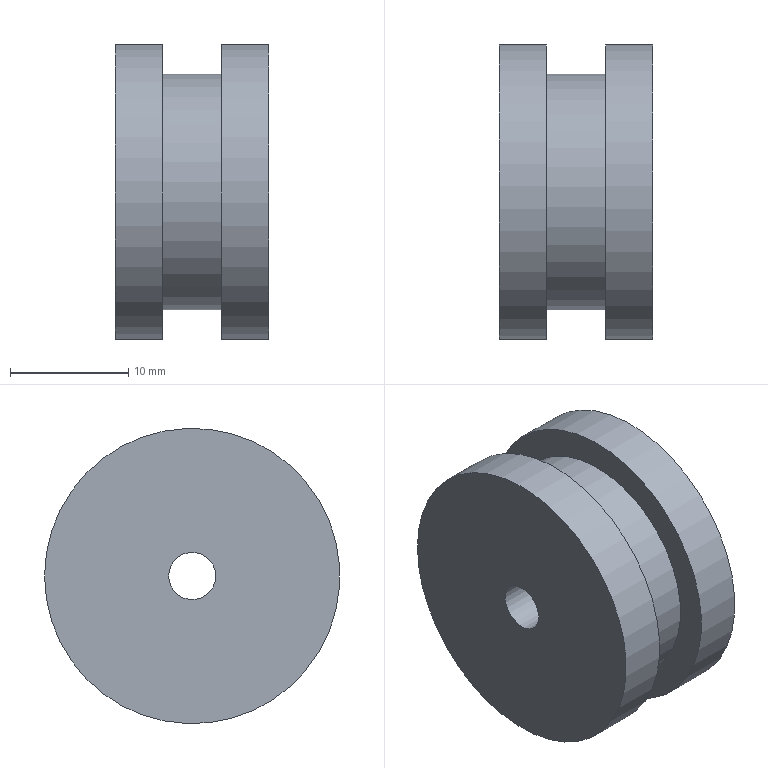Part | STEP file | 2-06.1 | 1 solid | 10 faces | box 13 x 25 x 25 mm | volume 5232 mm3 | cylinder 5 | plane 5 | commonest cylinder face diameters 25 x2 4 x1 6 x1 20 x1
STEP:
#1=CARTESIAN_POINT('',(0.,0.,0.));
#2=DIRECTION('',(0.,0.,1.));
#3=DIRECTION('',(1.,0.,0.));
#4=AXIS2_PLACEMENT_3D('',#1,#2,#3);
#5=CARTESIAN_POINT('',(2.5,10.,0.));
#6=VERTEX_POINT('',#5);
#7=CARTESIAN_POINT('',(-2.5,10.,0.));
#8=VERTEX_POINT('',#7);
#9=CARTESIAN_POINT('',(2.5,10.,0.));
#10=DIRECTION('',(-1.,0.,0.));
#11=VECTOR('',#10,1.);
#12=LINE('',#9,#11);
#13=CARTESIAN_POINT('',(2.5,0.,0.));
#14=DIRECTION('',(-1.,0.,0.));
#15=DIRECTION('',(0.,1.,0.));
#16=AXIS2_PLACEMENT_3D('',#13,#14,#15);
#17=CYLINDRICAL_SURFACE('',#16,10.);
#18=CARTESIAN_POINT('',(6.283,0.));
#19=DIRECTION('',(0.,1.));
#20=VECTOR('',#19,1.);
#21=LINE('',#18,#20);
#22=(GEOMETRIC_REPRESENTATION_CONTEXT(2)PARAMETRIC_REPRESENTATION_CONTEXT()REPRESENTATION_CONTEXT('',''));
#23=DEFINITIONAL_REPRESENTATION('',(#21),#22);
#24=PCURVE('',#17,#23);
#25=CARTESIAN_POINT('',(0.,0.));
#26=DIRECTION('',(0.,1.));
#27=VECTOR('',#26,1.);
#28=LINE('',#25,#27);
#29=(GEOMETRIC_REPRESENTATION_CONTEXT(2)PARAMETRIC_REPRESENTATION_CONTEXT()REPRESENTATION_CONTEXT('',''));
#30=DEFINITIONAL_REPRESENTATION('',(#28),#29);
#31=PCURVE('',#17,#30);
#32=SEAM_CURVE('',#12,(#24,#31),.PCURVE_S1.);
#33=EDGE_CURVE('',#6,#8,#32,.T.);
#34=ORIENTED_EDGE('',*,*,#33,.T.);
#35=CARTESIAN_POINT('',(-2.5,0.,0.));
#36=DIRECTION('',(1.,0.,0.));
#37=DIRECTION('',(0.,1.,0.));
#38=AXIS2_PLACEMENT_3D('',#35,#36,#37);
#39=CIRCLE('',#38,10.);
#40=CARTESIAN_POINT('',(6.283,5.));
#41=DIRECTION('',(-1.,0.));
#42=VECTOR('',#41,1.);
#43=LINE('',#40,#42);
#44=(GEOMETRIC_REPRESENTATION_CONTEXT(2)PARAMETRIC_REPRESENTATION_CONTEXT()REPRESENTATION_CONTEXT('',''));
#45=DEFINITIONAL_REPRESENTATION('',(#43),#44);
#46=PCURVE('',#17,#45);
#47=CARTESIAN_POINT('',(-2.5,-3.349,0.));
#48=DIRECTION('',(1.,0.,0.));
#49=DIRECTION('',(0.,0.,-1.));
#50=AXIS2_PLACEMENT_3D('',#47,#48,#49);
#51=PLANE('',#50);
#52=CARTESIAN_POINT('',(0.,3.349));
#53=DIRECTION('',(0.,1.));
#54=AXIS2_PLACEMENT_2D('',#52,#53);
#55=CIRCLE('',#54,10.);
#56=(GEOMETRIC_REPRESENTATION_CONTEXT(2)PARAMETRIC_REPRESENTATION_CONTEXT()REPRESENTATION_CONTEXT('',''));
#57=DEFINITIONAL_REPRESENTATION('',(#55),#56);
#58=PCURVE('',#51,#57);
#59=SURFACE_CURVE('',#39,(#46,#58),.PCURVE_S1.);
#60=EDGE_CURVE('',#8,#8,#59,.T.);
#61=ORIENTED_EDGE('',*,*,#60,.T.);
#62=ORIENTED_EDGE('',*,*,#33,.F.);
#63=CARTESIAN_POINT('',(2.5,0.,0.));
#64=DIRECTION('',(1.,0.,0.));
#65=DIRECTION('',(0.,1.,0.));
#66=AXIS2_PLACEMENT_3D('',#63,#64,#65);
#67=CIRCLE('',#66,10.);
#68=CARTESIAN_POINT('',(6.283,0.));
#69=DIRECTION('',(-1.,0.));
#70=VECTOR('',#69,1.);
#71=LINE('',#68,#70);
#72=(GEOMETRIC_REPRESENTATION_CONTEXT(2)PARAMETRIC_REPRESENTATION_CONTEXT()REPRESENTATION_CONTEXT('',''));
#73=DEFINITIONAL_REPRESENTATION('',(#71),#72);
#74=PCURVE('',#17,#73);
#75=CARTESIAN_POINT('',(2.5,-3.349,0.));
#76=DIRECTION('',(1.,0.,0.));
#77=DIRECTION('',(0.,0.,-1.));
#78=AXIS2_PLACEMENT_3D('',#75,#76,#77);
#79=PLANE('',#78);
#80=CARTESIAN_POINT('',(0.,3.349));
#81=DIRECTION('',(0.,1.));
#82=AXIS2_PLACEMENT_2D('',#80,#81);
#83=CIRCLE('',#82,10.);
#84=(GEOMETRIC_REPRESENTATION_CONTEXT(2)PARAMETRIC_REPRESENTATION_CONTEXT()REPRESENTATION_CONTEXT('',''));
#85=DEFINITIONAL_REPRESENTATION('',(#83),#84);
#86=PCURVE('',#79,#85);
#87=SURFACE_CURVE('',#67,(#74,#86),.PCURVE_S1.);
#88=EDGE_CURVE('',#6,#6,#87,.T.);
#89=ORIENTED_EDGE('',*,*,#88,.F.);
#90=EDGE_LOOP('',(#34,#61,#62,#89));
#91=FACE_BOUND('',#90,.T.);
#92=ADVANCED_FACE('',(#91),#17,.T.);
#93=CARTESIAN_POINT('',(-2.5,12.5,0.));
#94=VERTEX_POINT('',#93);
#95=CARTESIAN_POINT('',(-2.5,0.,0.));
#96=DIRECTION('',(1.,0.,0.));
#97=DIRECTION('',(0.,1.,0.));
#98=AXIS2_PLACEMENT_3D('',#95,#96,#97);
#99=CIRCLE('',#98,12.5);
#100=CARTESIAN_POINT('',(0.,3.349));
#101=DIRECTION('',(0.,1.));
#102=AXIS2_PLACEMENT_2D('',#100,#101);
#103=CIRCLE('',#102,12.5);
#104=(GEOMETRIC_REPRESENTATION_CONTEXT(2)PARAMETRIC_REPRESENTATION_CONTEXT()REPRESENTATION_CONTEXT('',''));
#105=DEFINITIONAL_REPRESENTATION('',(#103),#104);
#106=PCURVE('',#51,#105);
#107=CARTESIAN_POINT('',(-2.5,0.,0.));
#108=DIRECTION('',(-1.,0.,0.));
#109=DIRECTION('',(0.,1.,0.));
#110=AXIS2_PLACEMENT_3D('',#107,#108,#109);
#111=CYLINDRICAL_SURFACE('',#110,12.5);
#112=CARTESIAN_POINT('',(6.283,0.));
#113=DIRECTION('',(-1.,0.));
#114=VECTOR('',#113,1.);
#115=LINE('',#112,#114);
#116=(GEOMETRIC_REPRESENTATION_CONTEXT(2)PARAMETRIC_REPRESENTATION_CONTEXT()REPRESENTATION_CONTEXT('',''));
#117=DEFINITIONAL_REPRESENTATION('',(#115),#116);
#118=PCURVE('',#111,#117);
#119=SURFACE_CURVE('',#99,(#106,#118),.PCURVE_S1.);
#120=EDGE_CURVE('',#94,#94,#119,.T.);
#121=ORIENTED_EDGE('',*,*,#120,.T.);
#122=EDGE_LOOP('',(#121));
#123=FACE_BOUND('',#122,.T.);
#124=ORIENTED_EDGE('',*,*,#60,.F.);
#125=EDGE_LOOP('',(#124));
#126=FACE_BOUND('',#125,.T.);
#127=ADVANCED_FACE('',(#123,#126),#51,.T.);
#128=CARTESIAN_POINT('',(-6.5,12.5,0.));
#129=VERTEX_POINT('',#128);
#130=CARTESIAN_POINT('',(-2.5,12.5,0.));
#131=DIRECTION('',(-1.,0.,0.));
#132=VECTOR('',#131,1.);
#133=LINE('',#130,#132);
#134=CARTESIAN_POINT('',(6.283,0.));
#135=DIRECTION('',(0.,1.));
#136=VECTOR('',#135,1.);
#137=LINE('',#134,#136);
#138=(GEOMETRIC_REPRESENTATION_CONTEXT(2)PARAMETRIC_REPRESENTATION_CONTEXT()REPRESENTATION_CONTEXT('',''));
#139=DEFINITIONAL_REPRESENTATION('',(#137),#138);
#140=PCURVE('',#111,#139);
#141=CARTESIAN_POINT('',(0.,0.));
#142=DIRECTION('',(0.,1.));
#143=VECTOR('',#142,1.);
#144=LINE('',#141,#143);
#145=(GEOMETRIC_REPRESENTATION_CONTEXT(2)PARAMETRIC_REPRESENTATION_CONTEXT()REPRESENTATION_CONTEXT('',''));
#146=DEFINITIONAL_REPRESENTATION('',(#144),#145);
#147=PCURVE('',#111,#146);
#148=SEAM_CURVE('',#133,(#140,#147),.PCURVE_S1.);
#149=EDGE_CURVE('',#94,#129,#148,.T.);
#150=ORIENTED_EDGE('',*,*,#149,.T.);
#151=CARTESIAN_POINT('',(-6.5,0.,0.));
#152=DIRECTION('',(1.,0.,0.));
#153=DIRECTION('',(0.,1.,0.));
#154=AXIS2_PLACEMENT_3D('',#151,#152,#153);
#155=CIRCLE('',#154,12.5);
#156=CARTESIAN_POINT('',(6.283,4.));
#157=DIRECTION('',(-1.,0.));
#158=VECTOR('',#157,1.);
#159=LINE('',#156,#158);
#160=(GEOMETRIC_REPRESENTATION_CONTEXT(2)PARAMETRIC_REPRESENTATION_CONTEXT()REPRESENTATION_CONTEXT('',''));
#161=DEFINITIONAL_REPRESENTATION('',(#159),#160);
#162=PCURVE('',#111,#161);
#163=CARTESIAN_POINT('',(-6.5,-3.349,0.));
#164=DIRECTION('',(1.,0.,0.));
#165=DIRECTION('',(0.,0.,-1.));
#166=AXIS2_PLACEMENT_3D('',#163,#164,#165);
#167=PLANE('',#166);
#168=CARTESIAN_POINT('',(0.,3.349));
#169=DIRECTION('',(0.,1.));
#170=AXIS2_PLACEMENT_2D('',#168,#169);
#171=CIRCLE('',#170,12.5);
#172=(GEOMETRIC_REPRESENTATION_CONTEXT(2)PARAMETRIC_REPRESENTATION_CONTEXT()REPRESENTATION_CONTEXT('',''));
#173=DEFINITIONAL_REPRESENTATION('',(#171),#172);
#174=PCURVE('',#167,#173);
#175=SURFACE_CURVE('',#155,(#162,#174),.PCURVE_S1.);
#176=EDGE_CURVE('',#129,#129,#175,.T.);
#177=ORIENTED_EDGE('',*,*,#176,.T.);
#178=ORIENTED_EDGE('',*,*,#149,.F.);
#179=ORIENTED_EDGE('',*,*,#120,.F.);
#180=EDGE_LOOP('',(#150,#177,#178,#179));
#181=FACE_BOUND('',#180,.T.);
#182=ADVANCED_FACE('',(#181),#111,.T.);
#183=CARTESIAN_POINT('',(2.5,12.5,0.));
#184=VERTEX_POINT('',#183);
#185=CARTESIAN_POINT('',(2.5,0.,0.));
#186=DIRECTION('',(1.,0.,0.));
#187=DIRECTION('',(0.,1.,0.));
#188=AXIS2_PLACEMENT_3D('',#185,#186,#187);
#189=CIRCLE('',#188,12.5);
#190=CARTESIAN_POINT('',(0.,3.349));
#191=DIRECTION('',(0.,1.));
#192=AXIS2_PLACEMENT_2D('',#190,#191);
#193=CIRCLE('',#192,12.5);
#194=(GEOMETRIC_REPRESENTATION_CONTEXT(2)PARAMETRIC_REPRESENTATION_CONTEXT()REPRESENTATION_CONTEXT('',''));
#195=DEFINITIONAL_REPRESENTATION('',(#193),#194);
#196=PCURVE('',#79,#195);
#197=CARTESIAN_POINT('',(2.5,0.,0.));
#198=DIRECTION('',(1.,0.,0.));
#199=DIRECTION('',(0.,1.,0.));
#200=AXIS2_PLACEMENT_3D('',#197,#198,#199);
#201=CYLINDRICAL_SURFACE('',#200,12.5);
#202=CARTESIAN_POINT('',(0.,0.));
#203=DIRECTION('',(1.,0.));
#204=VECTOR('',#203,1.);
#205=LINE('',#202,#204);
#206=(GEOMETRIC_REPRESENTATION_CONTEXT(2)PARAMETRIC_REPRESENTATION_CONTEXT()REPRESENTATION_CONTEXT('',''));
#207=DEFINITIONAL_REPRESENTATION('',(#205),#206);
#208=PCURVE('',#201,#207);
#209=SURFACE_CURVE('',#189,(#196,#208),.PCURVE_S1.);
#210=EDGE_CURVE('',#184,#184,#209,.T.);
#211=ORIENTED_EDGE('',*,*,#210,.T.);
#212=EDGE_LOOP('',(#211));
#213=FACE_BOUND('',#212,.F.);
#214=ORIENTED_EDGE('',*,*,#88,.F.);
#215=EDGE_LOOP('',(#214));
#216=FACE_BOUND('',#215,.F.);
#217=ADVANCED_FACE('',(#213,#216),#79,.F.);
#218=ORIENTED_EDGE('',*,*,#210,.T.);
#219=CARTESIAN_POINT('',(6.5,12.5,0.));
#220=VERTEX_POINT('',#219);
#221=CARTESIAN_POINT('',(2.5,12.5,0.));
#222=DIRECTION('',(1.,0.,0.));
#223=VECTOR('',#222,1.);
#224=LINE('',#221,#223);
#225=CARTESIAN_POINT('',(6.283,0.));
#226=DIRECTION('',(0.,1.));
#227=VECTOR('',#226,1.);
#228=LINE('',#225,#227);
#229=(GEOMETRIC_REPRESENTATION_CONTEXT(2)PARAMETRIC_REPRESENTATION_CONTEXT()REPRESENTATION_CONTEXT('',''));
#230=DEFINITIONAL_REPRESENTATION('',(#228),#229);
#231=PCURVE('',#201,#230);
#232=CARTESIAN_POINT('',(0.,0.));
#233=DIRECTION('',(0.,1.));
#234=VECTOR('',#233,1.);
#235=LINE('',#232,#234);
#236=(GEOMETRIC_REPRESENTATION_CONTEXT(2)PARAMETRIC_REPRESENTATION_CONTEXT()REPRESENTATION_CONTEXT('',''));
#237=DEFINITIONAL_REPRESENTATION('',(#235),#236);
#238=PCURVE('',#201,#237);
#239=SEAM_CURVE('',#224,(#231,#238),.PCURVE_S1.);
#240=EDGE_CURVE('',#184,#220,#239,.T.);
#241=ORIENTED_EDGE('',*,*,#240,.T.);
#242=CARTESIAN_POINT('',(6.5,0.,0.));
#243=DIRECTION('',(1.,0.,0.));
#244=DIRECTION('',(0.,1.,0.));
#245=AXIS2_PLACEMENT_3D('',#242,#243,#244);
#246=CIRCLE('',#245,12.5);
#247=CARTESIAN_POINT('',(0.,4.));
#248=DIRECTION('',(1.,0.));
#249=VECTOR('',#248,1.);
#250=LINE('',#247,#249);
#251=(GEOMETRIC_REPRESENTATION_CONTEXT(2)PARAMETRIC_REPRESENTATION_CONTEXT()REPRESENTATION_CONTEXT('',''));
#252=DEFINITIONAL_REPRESENTATION('',(#250),#251);
#253=PCURVE('',#201,#252);
#254=CARTESIAN_POINT('',(6.5,-3.349,0.));
#255=DIRECTION('',(1.,0.,0.));
#256=DIRECTION('',(0.,0.,-1.));
#257=AXIS2_PLACEMENT_3D('',#254,#255,#256);
#258=PLANE('',#257);
#259=CARTESIAN_POINT('',(0.,3.349));
#260=DIRECTION('',(0.,1.));
#261=AXIS2_PLACEMENT_2D('',#259,#260);
#262=CIRCLE('',#261,12.5);
#263=(GEOMETRIC_REPRESENTATION_CONTEXT(2)PARAMETRIC_REPRESENTATION_CONTEXT()REPRESENTATION_CONTEXT('',''));
#264=DEFINITIONAL_REPRESENTATION('',(#262),#263);
#265=PCURVE('',#258,#264);
#266=SURFACE_CURVE('',#246,(#253,#265),.PCURVE_S1.);
#267=EDGE_CURVE('',#220,#220,#266,.T.);
#268=ORIENTED_EDGE('',*,*,#267,.F.);
#269=ORIENTED_EDGE('',*,*,#240,.F.);
#270=EDGE_LOOP('',(#218,#241,#268,#269));
#271=FACE_BOUND('',#270,.T.);
#272=ADVANCED_FACE('',(#271),#201,.T.);
#273=ORIENTED_EDGE('',*,*,#267,.T.);
#274=EDGE_LOOP('',(#273));
#275=FACE_BOUND('',#274,.T.);
#276=CARTESIAN_POINT('',(6.5,3.,0.));
#277=VERTEX_POINT('',#276);
#278=CARTESIAN_POINT('',(6.5,0.,0.));
#279=DIRECTION('',(1.,0.,0.));
#280=DIRECTION('',(0.,1.,0.));
#281=AXIS2_PLACEMENT_3D('',#278,#279,#280);
#282=CIRCLE('',#281,3.);
#283=CARTESIAN_POINT('',(0.,3.349));
#284=DIRECTION('',(0.,1.));
#285=AXIS2_PLACEMENT_2D('',#283,#284);
#286=CIRCLE('',#285,3.);
#287=(GEOMETRIC_REPRESENTATION_CONTEXT(2)PARAMETRIC_REPRESENTATION_CONTEXT()REPRESENTATION_CONTEXT('',''));
#288=DEFINITIONAL_REPRESENTATION('',(#286),#287);
#289=PCURVE('',#258,#288);
#290=CARTESIAN_POINT('',(6.5,0.,0.));
#291=DIRECTION('',(-1.,0.,0.));
#292=DIRECTION('',(0.,1.,0.));
#293=AXIS2_PLACEMENT_3D('',#290,#291,#292);
#294=CYLINDRICAL_SURFACE('',#293,3.);
#295=CARTESIAN_POINT('',(6.283,0.));
#296=DIRECTION('',(-1.,0.));
#297=VECTOR('',#296,1.);
#298=LINE('',#295,#297);
#299=(GEOMETRIC_REPRESENTATION_CONTEXT(2)PARAMETRIC_REPRESENTATION_CONTEXT()REPRESENTATION_CONTEXT('',''));
#300=DEFINITIONAL_REPRESENTATION('',(#298),#299);
#301=PCURVE('',#294,#300);
#302=SURFACE_CURVE('',#282,(#289,#301),.PCURVE_S1.);
#303=EDGE_CURVE('',#277,#277,#302,.T.);
#304=ORIENTED_EDGE('',*,*,#303,.F.);
#305=EDGE_LOOP('',(#304));
#306=FACE_BOUND('',#305,.T.);
#307=ADVANCED_FACE('',(#275,#306),#258,.T.);
#308=CARTESIAN_POINT('',(0.,3.,0.));
#309=VERTEX_POINT('',#308);
#310=CARTESIAN_POINT('',(6.5,3.,0.));
#311=DIRECTION('',(-1.,0.,0.));
#312=VECTOR('',#311,1.);
#313=LINE('',#310,#312);
#314=CARTESIAN_POINT('',(6.283,0.));
#315=DIRECTION('',(0.,1.));
#316=VECTOR('',#315,1.);
#317=LINE('',#314,#316);
#318=(GEOMETRIC_REPRESENTATION_CONTEXT(2)PARAMETRIC_REPRESENTATION_CONTEXT()REPRESENTATION_CONTEXT('',''));
#319=DEFINITIONAL_REPRESENTATION('',(#317),#318);
#320=PCURVE('',#294,#319);
#321=CARTESIAN_POINT('',(0.,0.));
#322=DIRECTION('',(0.,1.));
#323=VECTOR('',#322,1.);
#324=LINE('',#321,#323);
#325=(GEOMETRIC_REPRESENTATION_CONTEXT(2)PARAMETRIC_REPRESENTATION_CONTEXT()REPRESENTATION_CONTEXT('',''));
#326=DEFINITIONAL_REPRESENTATION('',(#324),#325);
#327=PCURVE('',#294,#326);
#328=SEAM_CURVE('',#313,(#320,#327),.PCURVE_S1.);
#329=EDGE_CURVE('',#277,#309,#328,.T.);
#330=ORIENTED_EDGE('',*,*,#329,.T.);
#331=CARTESIAN_POINT('',(0.,0.,0.));
#332=DIRECTION('',(1.,0.,0.));
#333=DIRECTION('',(0.,1.,0.));
#334=AXIS2_PLACEMENT_3D('',#331,#332,#333);
#335=CIRCLE('',#334,3.);
#336=CARTESIAN_POINT('',(6.283,6.5));
#337=DIRECTION('',(-1.,0.));
#338=VECTOR('',#337,1.);
#339=LINE('',#336,#338);
#340=(GEOMETRIC_REPRESENTATION_CONTEXT(2)PARAMETRIC_REPRESENTATION_CONTEXT()REPRESENTATION_CONTEXT('',''));
#341=DEFINITIONAL_REPRESENTATION('',(#339),#340);
#342=PCURVE('',#294,#341);
#343=CARTESIAN_POINT('',(0.,-0.8038,0.));
#344=DIRECTION('',(1.,0.,0.));
#345=DIRECTION('',(0.,0.,-1.));
#346=AXIS2_PLACEMENT_3D('',#343,#344,#345);
#347=PLANE('',#346);
#348=CARTESIAN_POINT('',(0.,0.8038));
#349=DIRECTION('',(0.,1.));
#350=AXIS2_PLACEMENT_2D('',#348,#349);
#351=CIRCLE('',#350,3.);
#352=(GEOMETRIC_REPRESENTATION_CONTEXT(2)PARAMETRIC_REPRESENTATION_CONTEXT()REPRESENTATION_CONTEXT('',''));
#353=DEFINITIONAL_REPRESENTATION('',(#351),#352);
#354=PCURVE('',#347,#353);
#355=SURFACE_CURVE('',#335,(#342,#354),.PCURVE_S1.);
#356=EDGE_CURVE('',#309,#309,#355,.T.);
#357=ORIENTED_EDGE('',*,*,#356,.T.);
#358=ORIENTED_EDGE('',*,*,#329,.F.);
#359=ORIENTED_EDGE('',*,*,#303,.F.);
#360=EDGE_LOOP('',(#330,#357,#358,#359));
#361=FACE_BOUND('',#360,.F.);
#362=ADVANCED_FACE('',(#361),#294,.F.);
#363=ORIENTED_EDGE('',*,*,#176,.T.);
#364=EDGE_LOOP('',(#363));
#365=FACE_BOUND('',#364,.F.);
#366=CARTESIAN_POINT('',(-6.5,2.,0.));
#367=VERTEX_POINT('',#366);
#368=CARTESIAN_POINT('',(-6.5,0.,0.));
#369=DIRECTION('',(-1.,0.,0.));
#370=DIRECTION('',(0.,1.,0.));
#371=AXIS2_PLACEMENT_3D('',#368,#369,#370);
#372=CIRCLE('',#371,2.);
#373=CARTESIAN_POINT('',(0.,5.349));
#374=CARTESIAN_POINT('',(3.464,5.349));
#375=CARTESIAN_POINT('',(1.732,2.349));
#376=CARTESIAN_POINT('',(0.,-0.6506));
#377=CARTESIAN_POINT('',(-1.732,2.349));
#378=CARTESIAN_POINT('',(-3.464,5.349));
#379=CARTESIAN_POINT('',(0.,5.349));
#380=(BOUNDED_CURVE()B_SPLINE_CURVE(2,(#373,#374,#375,#376,#377,#378,#379),.UNSPECIFIED.,.T.,.F.)B_SPLINE_CURVE_WITH_KNOTS((1,2,2,2,2,1),(-2.094,0.,2.094,4.189,6.283,8.378),.UNSPECIFIED.)CURVE()GEOMETRIC_REPRESENTATION_ITEM()RATIONAL_B_SPLINE_CURVE((1.,0.5,1.,0.5,1.,0.5,1.))REPRESENTATION_ITEM(''));
#381=(GEOMETRIC_REPRESENTATION_CONTEXT(2)PARAMETRIC_REPRESENTATION_CONTEXT()REPRESENTATION_CONTEXT('',''));
#382=DEFINITIONAL_REPRESENTATION('',(#380),#381);
#383=PCURVE('',#167,#382);
#384=CARTESIAN_POINT('',(0.,0.,0.));
#385=DIRECTION('',(-1.,0.,0.));
#386=DIRECTION('',(0.,1.,0.));
#387=AXIS2_PLACEMENT_3D('',#384,#385,#386);
#388=CYLINDRICAL_SURFACE('',#387,2.);
#389=CARTESIAN_POINT('',(0.,6.5));
#390=DIRECTION('',(1.,0.));
#391=VECTOR('',#390,1.);
#392=LINE('',#389,#391);
#393=(GEOMETRIC_REPRESENTATION_CONTEXT(2)PARAMETRIC_REPRESENTATION_CONTEXT()REPRESENTATION_CONTEXT('',''));
#394=DEFINITIONAL_REPRESENTATION('',(#392),#393);
#395=PCURVE('',#388,#394);
#396=SURFACE_CURVE('',#372,(#383,#395),.PCURVE_S1.);
#397=EDGE_CURVE('',#367,#367,#396,.T.);
#398=ORIENTED_EDGE('',*,*,#397,.T.);
#399=EDGE_LOOP('',(#398));
#400=FACE_BOUND('',#399,.F.);
#401=ADVANCED_FACE('',(#365,#400),#167,.F.);
#402=ORIENTED_EDGE('',*,*,#356,.T.);
#403=EDGE_LOOP('',(#402));
#404=FACE_BOUND('',#403,.T.);
#405=CARTESIAN_POINT('',(0.,2.,0.));
#406=VERTEX_POINT('',#405);
#407=CARTESIAN_POINT('',(0.,0.,0.));
#408=DIRECTION('',(1.,0.,0.));
#409=DIRECTION('',(0.,1.,0.));
#410=AXIS2_PLACEMENT_3D('',#407,#408,#409);
#411=CIRCLE('',#410,2.);
#412=CARTESIAN_POINT('',(0.,0.8038));
#413=DIRECTION('',(0.,1.));
#414=AXIS2_PLACEMENT_2D('',#412,#413);
#415=CIRCLE('',#414,2.);
#416=(GEOMETRIC_REPRESENTATION_CONTEXT(2)PARAMETRIC_REPRESENTATION_CONTEXT()REPRESENTATION_CONTEXT('',''));
#417=DEFINITIONAL_REPRESENTATION('',(#415),#416);
#418=PCURVE('',#347,#417);
#419=CARTESIAN_POINT('',(6.283,0.));
#420=DIRECTION('',(-1.,0.));
#421=VECTOR('',#420,1.);
#422=LINE('',#419,#421);
#423=(GEOMETRIC_REPRESENTATION_CONTEXT(2)PARAMETRIC_REPRESENTATION_CONTEXT()REPRESENTATION_CONTEXT('',''));
#424=DEFINITIONAL_REPRESENTATION('',(#422),#423);
#425=PCURVE('',#388,#424);
#426=SURFACE_CURVE('',#411,(#418,#425),.PCURVE_S1.);
#427=EDGE_CURVE('',#406,#406,#426,.T.);
#428=ORIENTED_EDGE('',*,*,#427,.F.);
#429=EDGE_LOOP('',(#428));
#430=FACE_BOUND('',#429,.T.);
#431=ADVANCED_FACE('',(#404,#430),#347,.T.);
#432=CARTESIAN_POINT('',(0.,2.,0.));
#433=DIRECTION('',(-1.,0.,0.));
#434=VECTOR('',#433,1.);
#435=LINE('',#432,#434);
#436=CARTESIAN_POINT('',(6.283,0.));
#437=DIRECTION('',(0.,1.));
#438=VECTOR('',#437,1.);
#439=LINE('',#436,#438);
#440=(GEOMETRIC_REPRESENTATION_CONTEXT(2)PARAMETRIC_REPRESENTATION_CONTEXT()REPRESENTATION_CONTEXT('',''));
#441=DEFINITIONAL_REPRESENTATION('',(#439),#440);
#442=PCURVE('',#388,#441);
#443=CARTESIAN_POINT('',(0.,0.));
#444=DIRECTION('',(0.,1.));
#445=VECTOR('',#444,1.);
#446=LINE('',#443,#445);
#447=(GEOMETRIC_REPRESENTATION_CONTEXT(2)PARAMETRIC_REPRESENTATION_CONTEXT()REPRESENTATION_CONTEXT('',''));
#448=DEFINITIONAL_REPRESENTATION('',(#446),#447);
#449=PCURVE('',#388,#448);
#450=SEAM_CURVE('',#435,(#442,#449),.PCURVE_S1.);
#451=EDGE_CURVE('',#406,#367,#450,.T.);
#452=ORIENTED_EDGE('',*,*,#451,.T.);
#453=ORIENTED_EDGE('',*,*,#397,.F.);
#454=ORIENTED_EDGE('',*,*,#451,.F.);
#455=ORIENTED_EDGE('',*,*,#427,.F.);
#456=EDGE_LOOP('',(#452,#453,#454,#455));
#457=FACE_BOUND('',#456,.F.);
#458=ADVANCED_FACE('',(#457),#388,.F.);
#459=CLOSED_SHELL('',(#92,#127,#182,#217,#272,#307,#362,#401,#431,#458));
#460=MANIFOLD_SOLID_BREP('',#459);
#461=(LENGTH_UNIT()NAMED_UNIT(*)SI_UNIT(.MILLI.,.METRE.));
#462=UNCERTAINTY_MEASURE_WITH_UNIT(LENGTH_MEASURE(0.0000001),#461,'','');
#463=(NAMED_UNIT(*)PLANE_ANGLE_UNIT()SI_UNIT($,.RADIAN.));
#464=(NAMED_UNIT(*)SI_UNIT($,.STERADIAN.)SOLID_ANGLE_UNIT());
#465=(GEOMETRIC_REPRESENTATION_CONTEXT(3)GLOBAL_UNCERTAINTY_ASSIGNED_CONTEXT((#462))GLOBAL_UNIT_ASSIGNED_CONTEXT((#461,#463,#464))REPRESENTATION_CONTEXT('',''));
#466=ADVANCED_BREP_SHAPE_REPRESENTATION('',(#4,#460),#465);